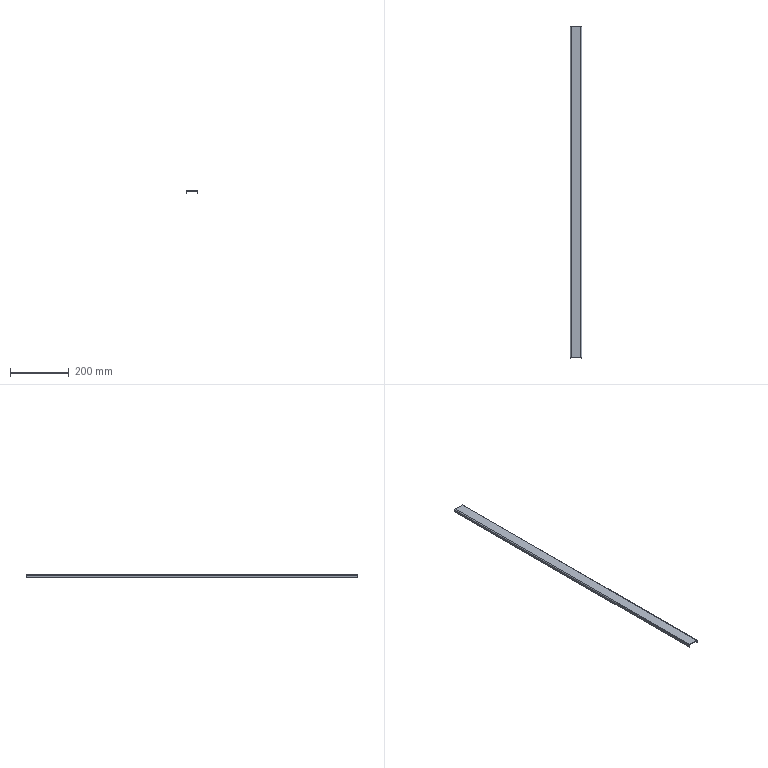Part | SolidWorks | features BaseBody 1 | 1 solid | 22 faces | box 40 x 1133 x 10 mm | volume 151532 mm3 | plane 18 | cylinder 4 | commonest cylinder face diameters 1 x2 6 x2
STEP:
#1=CARTESIAN_POINT('',(-17.5,566.5,-10.));
#2=VERTEX_POINT('',#1);
#3=CARTESIAN_POINT('',(-17.5,-566.5,-10.));
#4=VERTEX_POINT('',#3);
#5=CARTESIAN_POINT('',(-17.5,-566.5,-10.));
#6=DIRECTION('',(0.,-1.,0.));
#7=VECTOR('',#6,1000.);
#8=LINE('',#5,#7);
#9=EDGE_CURVE('',#2,#4,#8,.T.);
#10=ORIENTED_EDGE('',*,*,#9,.T.);
#11=CARTESIAN_POINT('',(-20.,-566.5,-10.));
#12=VERTEX_POINT('',#11);
#13=CARTESIAN_POINT('',(-20.,-566.5,-10.));
#14=DIRECTION('',(1.,0.,0.));
#15=VECTOR('',#14,1000.);
#16=LINE('',#13,#15);
#17=EDGE_CURVE('',#12,#4,#16,.T.);
#18=ORIENTED_EDGE('',*,*,#17,.F.);
#19=CARTESIAN_POINT('',(-20.,566.5,-10.));
#20=VERTEX_POINT('',#19);
#21=CARTESIAN_POINT('',(-20.,0.,-10.));
#22=DIRECTION('',(0.,-1.,0.));
#23=VECTOR('',#22,1000.);
#24=LINE('',#21,#23);
#25=EDGE_CURVE('',#20,#12,#24,.T.);
#26=ORIENTED_EDGE('',*,*,#25,.F.);
#27=CARTESIAN_POINT('',(-20.,566.5,-10.));
#28=DIRECTION('',(1.,0.,0.));
#29=VECTOR('',#28,1000.);
#30=LINE('',#27,#29);
#31=EDGE_CURVE('',#20,#2,#30,.T.);
#32=ORIENTED_EDGE('',*,*,#31,.T.);
#33=EDGE_LOOP('',(#10,#18,#26,#32));
#34=FACE_OUTER_BOUND('',#33,.T.);
#35=CARTESIAN_POINT('',(-20.,-566.5,-10.));
#36=DIRECTION('',(0.,0.,1.));
#37=DIRECTION('',(1.,0.,0.));
#38=AXIS2_PLACEMENT_3D('',#35,#36,#37);
#39=PLANE('',#38);
#40=ADVANCED_FACE('',(#34),#39,.F.);
#41=CARTESIAN_POINT('',(-17.5,566.5,-3.));
#42=VERTEX_POINT('',#41);
#43=CARTESIAN_POINT('',(-17.5,566.5,-10.));
#44=DIRECTION('',(0.,0.,-1.));
#45=VECTOR('',#44,1000.);
#46=LINE('',#43,#45);
#47=EDGE_CURVE('',#42,#2,#46,.T.);
#48=ORIENTED_EDGE('',*,*,#47,.F.);
#49=CARTESIAN_POINT('',(-17.5,-566.5,-3.));
#50=VERTEX_POINT('',#49);
#51=CARTESIAN_POINT('',(-17.5,-566.5,-3.));
#52=DIRECTION('',(0.,1.,0.));
#53=VECTOR('',#52,1000.);
#54=LINE('',#51,#53);
#55=EDGE_CURVE('',#50,#42,#54,.T.);
#56=ORIENTED_EDGE('',*,*,#55,.F.);
#57=CARTESIAN_POINT('',(-17.5,-566.5,-2.5));
#58=DIRECTION('',(0.,0.,1.));
#59=VECTOR('',#58,1000.);
#60=LINE('',#57,#59);
#61=EDGE_CURVE('',#4,#50,#60,.T.);
#62=ORIENTED_EDGE('',*,*,#61,.F.);
#63=ORIENTED_EDGE('',*,*,#9,.F.);
#64=EDGE_LOOP('',(#48,#56,#62,#63));
#65=FACE_OUTER_BOUND('',#64,.T.);
#66=CARTESIAN_POINT('',(-17.5,0.,0.));
#67=DIRECTION('',(1.,0.,0.));
#68=DIRECTION('',(0.,0.,-1.));
#69=AXIS2_PLACEMENT_3D('',#66,#67,#68);
#70=PLANE('',#69);
#71=ADVANCED_FACE('',(#65),#70,.T.);
#72=CARTESIAN_POINT('',(-20.,566.5,-3.));
#73=VERTEX_POINT('',#72);
#74=CARTESIAN_POINT('',(-20.,-566.5,-3.));
#75=VERTEX_POINT('',#74);
#76=CARTESIAN_POINT('',(-20.,-566.5,-3.));
#77=DIRECTION('',(0.,-1.,0.));
#78=VECTOR('',#77,1000.);
#79=LINE('',#76,#78);
#80=EDGE_CURVE('',#73,#75,#79,.T.);
#81=ORIENTED_EDGE('',*,*,#80,.F.);
#82=CARTESIAN_POINT('',(-20.,566.5,0.));
#83=DIRECTION('',(0.,0.,-1.));
#84=VECTOR('',#83,1000.);
#85=LINE('',#82,#84);
#86=EDGE_CURVE('',#73,#20,#85,.T.);
#87=ORIENTED_EDGE('',*,*,#86,.T.);
#88=ORIENTED_EDGE('',*,*,#25,.T.);
#89=CARTESIAN_POINT('',(-20.,-566.5,0.));
#90=DIRECTION('',(0.,0.,1.));
#91=VECTOR('',#90,1000.);
#92=LINE('',#89,#91);
#93=EDGE_CURVE('',#12,#75,#92,.T.);
#94=ORIENTED_EDGE('',*,*,#93,.T.);
#95=EDGE_LOOP('',(#81,#87,#88,#94));
#96=FACE_OUTER_BOUND('',#95,.T.);
#97=CARTESIAN_POINT('',(-20.,0.,0.));
#98=DIRECTION('',(1.,0.,0.));
#99=DIRECTION('',(0.,0.,-1.));
#100=AXIS2_PLACEMENT_3D('',#97,#98,#99);
#101=PLANE('',#100);
#102=ADVANCED_FACE('',(#96),#101,.F.);
#103=CARTESIAN_POINT('',(-20.,-566.5,-3.));
#104=DIRECTION('',(-1.,0.,0.));
#105=VECTOR('',#104,1000.);
#106=LINE('',#103,#105);
#107=EDGE_CURVE('',#50,#75,#106,.T.);
#108=ORIENTED_EDGE('',*,*,#107,.T.);
#109=ORIENTED_EDGE('',*,*,#93,.F.);
#110=ORIENTED_EDGE('',*,*,#17,.T.);
#111=ORIENTED_EDGE('',*,*,#61,.T.);
#112=EDGE_LOOP('',(#108,#109,#110,#111));
#113=FACE_OUTER_BOUND('',#112,.T.);
#114=CARTESIAN_POINT('',(-20.,-566.5,-2.5));
#115=DIRECTION('',(0.,1.,0.));
#116=DIRECTION('',(0.,0.,-1.));
#117=AXIS2_PLACEMENT_3D('',#114,#115,#116);
#118=PLANE('',#117);
#119=ADVANCED_FACE('',(#113),#118,.F.);
#120=CARTESIAN_POINT('',(-17.5,566.5,-3.));
#121=DIRECTION('',(-1.,0.,0.));
#122=VECTOR('',#121,1000.);
#123=LINE('',#120,#122);
#124=EDGE_CURVE('',#42,#73,#123,.T.);
#125=ORIENTED_EDGE('',*,*,#124,.F.);
#126=ORIENTED_EDGE('',*,*,#47,.T.);
#127=ORIENTED_EDGE('',*,*,#31,.F.);
#128=ORIENTED_EDGE('',*,*,#86,.F.);
#129=EDGE_LOOP('',(#125,#126,#127,#128));
#130=FACE_OUTER_BOUND('',#129,.T.);
#131=CARTESIAN_POINT('',(-20.,566.5,-10.));
#132=DIRECTION('',(0.,-1.,0.));
#133=DIRECTION('',(0.,0.,-1.));
#134=AXIS2_PLACEMENT_3D('',#131,#132,#133);
#135=PLANE('',#134);
#136=ADVANCED_FACE('',(#130),#135,.F.);
#137=CARTESIAN_POINT('',(-17.,566.5,-2.5));
#138=VERTEX_POINT('',#137);
#139=CARTESIAN_POINT('',(-17.,-566.5,-2.5));
#140=VERTEX_POINT('',#139);
#141=CARTESIAN_POINT('',(-17.,566.5,-2.5));
#142=DIRECTION('',(0.,-1.,0.));
#143=VECTOR('',#142,1000.);
#144=LINE('',#141,#143);
#145=EDGE_CURVE('',#138,#140,#144,.T.);
#146=ORIENTED_EDGE('',*,*,#145,.T.);
#147=CARTESIAN_POINT('',(-17.,-566.5,-3.));
#148=DIRECTION('',(0.,-1.,0.));
#149=DIRECTION('',(0.,0.,1.));
#150=AXIS2_PLACEMENT_3D('',#147,#148,#149);
#151=CIRCLE('',#150,0.5);
#152=EDGE_CURVE('',#140,#50,#151,.T.);
#153=ORIENTED_EDGE('',*,*,#152,.T.);
#154=ORIENTED_EDGE('',*,*,#55,.T.);
#155=CARTESIAN_POINT('',(-17.,566.5,-3.));
#156=DIRECTION('',(0.,1.,0.));
#157=DIRECTION('',(0.,0.,1.));
#158=AXIS2_PLACEMENT_3D('',#155,#156,#157);
#159=CIRCLE('',#158,0.5);
#160=EDGE_CURVE('',#42,#138,#159,.T.);
#161=ORIENTED_EDGE('',*,*,#160,.T.);
#162=EDGE_LOOP('',(#146,#153,#154,#161));
#163=FACE_OUTER_BOUND('',#162,.T.);
#164=CARTESIAN_POINT('',(-17.,566.5,-3.));
#165=DIRECTION('',(0.,1.,0.));
#166=DIRECTION('',(-1.,0.,0.));
#167=AXIS2_PLACEMENT_3D('',#164,#165,#166);
#168=CYLINDRICAL_SURFACE('',#167,0.5);
#169=ADVANCED_FACE('',(#163),#168,.F.);
#170=CARTESIAN_POINT('',(-17.,566.5,0.));
#171=VERTEX_POINT('',#170);
#172=CARTESIAN_POINT('',(-17.,-566.5,0.));
#173=VERTEX_POINT('',#172);
#174=CARTESIAN_POINT('',(-17.,566.5,0.));
#175=DIRECTION('',(0.,-1.,0.));
#176=VECTOR('',#175,1000.);
#177=LINE('',#174,#176);
#178=EDGE_CURVE('',#171,#173,#177,.T.);
#179=ORIENTED_EDGE('',*,*,#178,.F.);
#180=CARTESIAN_POINT('',(-17.,566.5,-3.));
#181=DIRECTION('',(0.,1.,0.));
#182=DIRECTION('',(0.,0.,1.));
#183=AXIS2_PLACEMENT_3D('',#180,#181,#182);
#184=CIRCLE('',#183,3.);
#185=EDGE_CURVE('',#73,#171,#184,.T.);
#186=ORIENTED_EDGE('',*,*,#185,.F.);
#187=ORIENTED_EDGE('',*,*,#80,.T.);
#188=CARTESIAN_POINT('',(-17.,-566.5,-3.));
#189=DIRECTION('',(0.,-1.,0.));
#190=DIRECTION('',(0.,0.,1.));
#191=AXIS2_PLACEMENT_3D('',#188,#189,#190);
#192=CIRCLE('',#191,3.);
#193=EDGE_CURVE('',#173,#75,#192,.T.);
#194=ORIENTED_EDGE('',*,*,#193,.F.);
#195=EDGE_LOOP('',(#179,#186,#187,#194));
#196=FACE_OUTER_BOUND('',#195,.T.);
#197=CARTESIAN_POINT('',(-17.,566.5,-3.));
#198=DIRECTION('',(0.,1.,0.));
#199=DIRECTION('',(-1.,0.,0.));
#200=AXIS2_PLACEMENT_3D('',#197,#198,#199);
#201=CYLINDRICAL_SURFACE('',#200,3.);
#202=ADVANCED_FACE('',(#196),#201,.T.);
#203=ORIENTED_EDGE('',*,*,#160,.F.);
#204=ORIENTED_EDGE('',*,*,#124,.T.);
#205=ORIENTED_EDGE('',*,*,#185,.T.);
#206=CARTESIAN_POINT('',(-17.,566.5,-2.5));
#207=DIRECTION('',(0.,0.,1.));
#208=VECTOR('',#207,1000.);
#209=LINE('',#206,#208);
#210=EDGE_CURVE('',#138,#171,#209,.T.);
#211=ORIENTED_EDGE('',*,*,#210,.F.);
#212=EDGE_LOOP('',(#203,#204,#205,#211));
#213=FACE_OUTER_BOUND('',#212,.T.);
#214=CARTESIAN_POINT('',(-17.,566.5,-3.));
#215=DIRECTION('',(0.,-1.,0.));
#216=DIRECTION('',(0.,0.,-1.));
#217=AXIS2_PLACEMENT_3D('',#214,#215,#216);
#218=PLANE('',#217);
#219=ADVANCED_FACE('',(#213),#218,.F.);
#220=ORIENTED_EDGE('',*,*,#107,.F.);
#221=ORIENTED_EDGE('',*,*,#152,.F.);
#222=CARTESIAN_POINT('',(-17.,-566.5,-2.5));
#223=DIRECTION('',(0.,0.,1.));
#224=VECTOR('',#223,1000.);
#225=LINE('',#222,#224);
#226=EDGE_CURVE('',#140,#173,#225,.T.);
#227=ORIENTED_EDGE('',*,*,#226,.T.);
#228=ORIENTED_EDGE('',*,*,#193,.T.);
#229=EDGE_LOOP('',(#220,#221,#227,#228));
#230=FACE_OUTER_BOUND('',#229,.T.);
#231=CARTESIAN_POINT('',(-17.,-566.5,-3.));
#232=DIRECTION('',(0.,-1.,0.));
#233=DIRECTION('',(0.,0.,-1.));
#234=AXIS2_PLACEMENT_3D('',#231,#232,#233);
#235=PLANE('',#234);
#236=ADVANCED_FACE('',(#230),#235,.T.);
#237=CARTESIAN_POINT('',(17.5,-566.5,-10.));
#238=VERTEX_POINT('',#237);
#239=CARTESIAN_POINT('',(17.5,566.5,-10.));
#240=VERTEX_POINT('',#239);
#241=CARTESIAN_POINT('',(17.5,566.5,-10.));
#242=DIRECTION('',(0.,1.,0.));
#243=VECTOR('',#242,1000.);
#244=LINE('',#241,#243);
#245=EDGE_CURVE('',#238,#240,#244,.T.);
#246=ORIENTED_EDGE('',*,*,#245,.T.);
#247=CARTESIAN_POINT('',(20.,566.5,-10.));
#248=VERTEX_POINT('',#247);
#249=CARTESIAN_POINT('',(20.,566.5,-10.));
#250=DIRECTION('',(-1.,0.,0.));
#251=VECTOR('',#250,1000.);
#252=LINE('',#249,#251);
#253=EDGE_CURVE('',#248,#240,#252,.T.);
#254=ORIENTED_EDGE('',*,*,#253,.F.);
#255=CARTESIAN_POINT('',(20.,-566.5,-10.));
#256=VERTEX_POINT('',#255);
#257=CARTESIAN_POINT('',(20.,0.,-10.));
#258=DIRECTION('',(0.,1.,0.));
#259=VECTOR('',#258,1000.);
#260=LINE('',#257,#259);
#261=EDGE_CURVE('',#256,#248,#260,.T.);
#262=ORIENTED_EDGE('',*,*,#261,.F.);
#263=CARTESIAN_POINT('',(20.,-566.5,-10.));
#264=DIRECTION('',(-1.,0.,0.));
#265=VECTOR('',#264,1000.);
#266=LINE('',#263,#265);
#267=EDGE_CURVE('',#256,#238,#266,.T.);
#268=ORIENTED_EDGE('',*,*,#267,.T.);
#269=EDGE_LOOP('',(#246,#254,#262,#268));
#270=FACE_OUTER_BOUND('',#269,.T.);
#271=CARTESIAN_POINT('',(20.,566.5,-10.));
#272=DIRECTION('',(0.,0.,1.));
#273=DIRECTION('',(1.,0.,0.));
#274=AXIS2_PLACEMENT_3D('',#271,#272,#273);
#275=PLANE('',#274);
#276=ADVANCED_FACE('',(#270),#275,.F.);
#277=CARTESIAN_POINT('',(17.5,-566.5,-3.));
#278=VERTEX_POINT('',#277);
#279=CARTESIAN_POINT('',(17.5,-566.5,-10.));
#280=DIRECTION('',(0.,0.,-1.));
#281=VECTOR('',#280,1000.);
#282=LINE('',#279,#281);
#283=EDGE_CURVE('',#278,#238,#282,.T.);
#284=ORIENTED_EDGE('',*,*,#283,.F.);
#285=CARTESIAN_POINT('',(17.5,566.5,-3.));
#286=VERTEX_POINT('',#285);
#287=CARTESIAN_POINT('',(17.5,566.5,-3.));
#288=DIRECTION('',(0.,-1.,0.));
#289=VECTOR('',#288,1000.);
#290=LINE('',#287,#289);
#291=EDGE_CURVE('',#286,#278,#290,.T.);
#292=ORIENTED_EDGE('',*,*,#291,.F.);
#293=CARTESIAN_POINT('',(17.5,566.5,-2.5));
#294=DIRECTION('',(0.,0.,1.));
#295=VECTOR('',#294,1000.);
#296=LINE('',#293,#295);
#297=EDGE_CURVE('',#240,#286,#296,.T.);
#298=ORIENTED_EDGE('',*,*,#297,.F.);
#299=ORIENTED_EDGE('',*,*,#245,.F.);
#300=EDGE_LOOP('',(#284,#292,#298,#299));
#301=FACE_OUTER_BOUND('',#300,.T.);
#302=CARTESIAN_POINT('',(17.5,0.,0.));
#303=DIRECTION('',(-1.,0.,0.));
#304=DIRECTION('',(0.,0.,1.));
#305=AXIS2_PLACEMENT_3D('',#302,#303,#304);
#306=PLANE('',#305);
#307=ADVANCED_FACE('',(#301),#306,.T.);
#308=CARTESIAN_POINT('',(20.,-566.5,-3.));
#309=VERTEX_POINT('',#308);
#310=CARTESIAN_POINT('',(20.,566.5,-3.));
#311=VERTEX_POINT('',#310);
#312=CARTESIAN_POINT('',(20.,566.5,-3.));
#313=DIRECTION('',(0.,1.,0.));
#314=VECTOR('',#313,1000.);
#315=LINE('',#312,#314);
#316=EDGE_CURVE('',#309,#311,#315,.T.);
#317=ORIENTED_EDGE('',*,*,#316,.F.);
#318=CARTESIAN_POINT('',(20.,-566.5,0.));
#319=DIRECTION('',(0.,0.,-1.));
#320=VECTOR('',#319,1000.);
#321=LINE('',#318,#320);
#322=EDGE_CURVE('',#309,#256,#321,.T.);
#323=ORIENTED_EDGE('',*,*,#322,.T.);
#324=ORIENTED_EDGE('',*,*,#261,.T.);
#325=CARTESIAN_POINT('',(20.,566.5,0.));
#326=DIRECTION('',(0.,0.,1.));
#327=VECTOR('',#326,1000.);
#328=LINE('',#325,#327);
#329=EDGE_CURVE('',#248,#311,#328,.T.);
#330=ORIENTED_EDGE('',*,*,#329,.T.);
#331=EDGE_LOOP('',(#317,#323,#324,#330));
#332=FACE_OUTER_BOUND('',#331,.T.);
#333=CARTESIAN_POINT('',(20.,0.,0.));
#334=DIRECTION('',(-1.,0.,0.));
#335=DIRECTION('',(0.,0.,1.));
#336=AXIS2_PLACEMENT_3D('',#333,#334,#335);
#337=PLANE('',#336);
#338=ADVANCED_FACE('',(#332),#337,.F.);
#339=CARTESIAN_POINT('',(20.,566.5,-3.));
#340=DIRECTION('',(1.,0.,0.));
#341=VECTOR('',#340,1000.);
#342=LINE('',#339,#341);
#343=EDGE_CURVE('',#286,#311,#342,.T.);
#344=ORIENTED_EDGE('',*,*,#343,.T.);
#345=ORIENTED_EDGE('',*,*,#329,.F.);
#346=ORIENTED_EDGE('',*,*,#253,.T.);
#347=ORIENTED_EDGE('',*,*,#297,.T.);
#348=EDGE_LOOP('',(#344,#345,#346,#347));
#349=FACE_OUTER_BOUND('',#348,.T.);
#350=CARTESIAN_POINT('',(20.,566.5,-2.5));
#351=DIRECTION('',(0.,-1.,0.));
#352=DIRECTION('',(0.,0.,-1.));
#353=AXIS2_PLACEMENT_3D('',#350,#351,#352);
#354=PLANE('',#353);
#355=ADVANCED_FACE('',(#349),#354,.F.);
#356=CARTESIAN_POINT('',(17.5,-566.5,-3.));
#357=DIRECTION('',(1.,0.,0.));
#358=VECTOR('',#357,1000.);
#359=LINE('',#356,#358);
#360=EDGE_CURVE('',#278,#309,#359,.T.);
#361=ORIENTED_EDGE('',*,*,#360,.F.);
#362=ORIENTED_EDGE('',*,*,#283,.T.);
#363=ORIENTED_EDGE('',*,*,#267,.F.);
#364=ORIENTED_EDGE('',*,*,#322,.F.);
#365=EDGE_LOOP('',(#361,#362,#363,#364));
#366=FACE_OUTER_BOUND('',#365,.T.);
#367=CARTESIAN_POINT('',(20.,-566.5,-10.));
#368=DIRECTION('',(0.,1.,0.));
#369=DIRECTION('',(0.,0.,-1.));
#370=AXIS2_PLACEMENT_3D('',#367,#368,#369);
#371=PLANE('',#370);
#372=ADVANCED_FACE('',(#366),#371,.F.);
#373=CARTESIAN_POINT('',(17.,-566.5,-2.5));
#374=VERTEX_POINT('',#373);
#375=CARTESIAN_POINT('',(17.,566.5,-2.5));
#376=VERTEX_POINT('',#375);
#377=CARTESIAN_POINT('',(17.,-566.5,-2.5));
#378=DIRECTION('',(0.,1.,0.));
#379=VECTOR('',#378,1000.);
#380=LINE('',#377,#379);
#381=EDGE_CURVE('',#374,#376,#380,.T.);
#382=ORIENTED_EDGE('',*,*,#381,.T.);
#383=CARTESIAN_POINT('',(17.,566.5,-3.));
#384=DIRECTION('',(0.,1.,0.));
#385=DIRECTION('',(0.,0.,-1.));
#386=AXIS2_PLACEMENT_3D('',#383,#384,#385);
#387=CIRCLE('',#386,0.5);
#388=EDGE_CURVE('',#376,#286,#387,.T.);
#389=ORIENTED_EDGE('',*,*,#388,.T.);
#390=ORIENTED_EDGE('',*,*,#291,.T.);
#391=CARTESIAN_POINT('',(17.,-566.5,-3.));
#392=DIRECTION('',(0.,-1.,0.));
#393=DIRECTION('',(0.,0.,-1.));
#394=AXIS2_PLACEMENT_3D('',#391,#392,#393);
#395=CIRCLE('',#394,0.5);
#396=EDGE_CURVE('',#278,#374,#395,.T.);
#397=ORIENTED_EDGE('',*,*,#396,.T.);
#398=EDGE_LOOP('',(#382,#389,#390,#397));
#399=FACE_OUTER_BOUND('',#398,.T.);
#400=CARTESIAN_POINT('',(17.,-566.5,-3.));
#401=DIRECTION('',(0.,-1.,0.));
#402=DIRECTION('',(1.,0.,0.));
#403=AXIS2_PLACEMENT_3D('',#400,#401,#402);
#404=CYLINDRICAL_SURFACE('',#403,0.5);
#405=ADVANCED_FACE('',(#399),#404,.F.);
#406=CARTESIAN_POINT('',(17.,-566.5,0.));
#407=VERTEX_POINT('',#406);
#408=CARTESIAN_POINT('',(17.,566.5,0.));
#409=VERTEX_POINT('',#408);
#410=CARTESIAN_POINT('',(17.,-566.5,0.));
#411=DIRECTION('',(0.,1.,0.));
#412=VECTOR('',#411,1000.);
#413=LINE('',#410,#412);
#414=EDGE_CURVE('',#407,#409,#413,.T.);
#415=ORIENTED_EDGE('',*,*,#414,.F.);
#416=CARTESIAN_POINT('',(17.,-566.5,-3.));
#417=DIRECTION('',(0.,-1.,0.));
#418=DIRECTION('',(0.,0.,-1.));
#419=AXIS2_PLACEMENT_3D('',#416,#417,#418);
#420=CIRCLE('',#419,3.);
#421=EDGE_CURVE('',#309,#407,#420,.T.);
#422=ORIENTED_EDGE('',*,*,#421,.F.);
#423=ORIENTED_EDGE('',*,*,#316,.T.);
#424=CARTESIAN_POINT('',(17.,566.5,-3.));
#425=DIRECTION('',(0.,1.,0.));
#426=DIRECTION('',(0.,0.,-1.));
#427=AXIS2_PLACEMENT_3D('',#424,#425,#426);
#428=CIRCLE('',#427,3.);
#429=EDGE_CURVE('',#409,#311,#428,.T.);
#430=ORIENTED_EDGE('',*,*,#429,.F.);
#431=EDGE_LOOP('',(#415,#422,#423,#430));
#432=FACE_OUTER_BOUND('',#431,.T.);
#433=CARTESIAN_POINT('',(17.,-566.5,-3.));
#434=DIRECTION('',(0.,-1.,0.));
#435=DIRECTION('',(1.,0.,0.));
#436=AXIS2_PLACEMENT_3D('',#433,#434,#435);
#437=CYLINDRICAL_SURFACE('',#436,3.);
#438=ADVANCED_FACE('',(#432),#437,.T.);
#439=ORIENTED_EDGE('',*,*,#396,.F.);
#440=ORIENTED_EDGE('',*,*,#360,.T.);
#441=ORIENTED_EDGE('',*,*,#421,.T.);
#442=CARTESIAN_POINT('',(17.,-566.5,-2.5));
#443=DIRECTION('',(0.,0.,1.));
#444=VECTOR('',#443,1000.);
#445=LINE('',#442,#444);
#446=EDGE_CURVE('',#374,#407,#445,.T.);
#447=ORIENTED_EDGE('',*,*,#446,.F.);
#448=EDGE_LOOP('',(#439,#440,#441,#447));
#449=FACE_OUTER_BOUND('',#448,.T.);
#450=CARTESIAN_POINT('',(17.,-566.5,-3.));
#451=DIRECTION('',(0.,1.,0.));
#452=DIRECTION('',(1.,0.,0.));
#453=AXIS2_PLACEMENT_3D('',#450,#451,#452);
#454=PLANE('',#453);
#455=ADVANCED_FACE('',(#449),#454,.F.);
#456=ORIENTED_EDGE('',*,*,#343,.F.);
#457=ORIENTED_EDGE('',*,*,#388,.F.);
#458=CARTESIAN_POINT('',(17.,566.5,-2.5));
#459=DIRECTION('',(0.,0.,1.));
#460=VECTOR('',#459,1000.);
#461=LINE('',#458,#460);
#462=EDGE_CURVE('',#376,#409,#461,.T.);
#463=ORIENTED_EDGE('',*,*,#462,.T.);
#464=ORIENTED_EDGE('',*,*,#429,.T.);
#465=EDGE_LOOP('',(#456,#457,#463,#464));
#466=FACE_OUTER_BOUND('',#465,.T.);
#467=CARTESIAN_POINT('',(17.,566.5,-3.));
#468=DIRECTION('',(0.,1.,0.));
#469=DIRECTION('',(1.,0.,0.));
#470=AXIS2_PLACEMENT_3D('',#467,#468,#469);
#471=PLANE('',#470);
#472=ADVANCED_FACE('',(#466),#471,.T.);
#473=ORIENTED_EDGE('',*,*,#226,.F.);
#474=CARTESIAN_POINT('',(20.,-566.5,-2.5));
#475=DIRECTION('',(1.,0.,0.));
#476=VECTOR('',#475,1000.);
#477=LINE('',#474,#476);
#478=EDGE_CURVE('',#140,#374,#477,.T.);
#479=ORIENTED_EDGE('',*,*,#478,.T.);
#480=ORIENTED_EDGE('',*,*,#446,.T.);
#481=CARTESIAN_POINT('',(20.,-566.5,0.));
#482=DIRECTION('',(1.,0.,0.));
#483=VECTOR('',#482,1000.);
#484=LINE('',#481,#483);
#485=EDGE_CURVE('',#173,#407,#484,.T.);
#486=ORIENTED_EDGE('',*,*,#485,.F.);
#487=EDGE_LOOP('',(#473,#479,#480,#486));
#488=FACE_OUTER_BOUND('',#487,.T.);
#489=CARTESIAN_POINT('',(20.,-566.5,-2.5));
#490=DIRECTION('',(0.,-1.,0.));
#491=DIRECTION('',(0.,0.,-1.));
#492=AXIS2_PLACEMENT_3D('',#489,#490,#491);
#493=PLANE('',#492);
#494=ADVANCED_FACE('',(#488),#493,.T.);
#495=CARTESIAN_POINT('',(20.,566.5,-2.5));
#496=DIRECTION('',(-1.,0.,0.));
#497=VECTOR('',#496,1000.);
#498=LINE('',#495,#497);
#499=EDGE_CURVE('',#376,#138,#498,.T.);
#500=ORIENTED_EDGE('',*,*,#499,.T.);
#501=ORIENTED_EDGE('',*,*,#210,.T.);
#502=CARTESIAN_POINT('',(20.,566.5,0.));
#503=DIRECTION('',(-1.,0.,0.));
#504=VECTOR('',#503,1000.);
#505=LINE('',#502,#504);
#506=EDGE_CURVE('',#409,#171,#505,.T.);
#507=ORIENTED_EDGE('',*,*,#506,.F.);
#508=ORIENTED_EDGE('',*,*,#462,.F.);
#509=EDGE_LOOP('',(#500,#501,#507,#508));
#510=FACE_OUTER_BOUND('',#509,.T.);
#511=CARTESIAN_POINT('',(20.,566.5,-2.5));
#512=DIRECTION('',(0.,1.,0.));
#513=DIRECTION('',(1.,0.,0.));
#514=AXIS2_PLACEMENT_3D('',#511,#512,#513);
#515=PLANE('',#514);
#516=ADVANCED_FACE('',(#510),#515,.T.);
#517=ORIENTED_EDGE('',*,*,#178,.T.);
#518=ORIENTED_EDGE('',*,*,#485,.T.);
#519=ORIENTED_EDGE('',*,*,#414,.T.);
#520=ORIENTED_EDGE('',*,*,#506,.T.);
#521=EDGE_LOOP('',(#517,#518,#519,#520));
#522=FACE_OUTER_BOUND('',#521,.T.);
#523=CARTESIAN_POINT('',(0.,0.,0.));
#524=DIRECTION('',(0.,0.,-1.));
#525=DIRECTION('',(0.,-1.,0.));
#526=AXIS2_PLACEMENT_3D('',#523,#524,#525);
#527=PLANE('',#526);
#528=ADVANCED_FACE('',(#522),#527,.F.);
#529=ORIENTED_EDGE('',*,*,#478,.F.);
#530=ORIENTED_EDGE('',*,*,#145,.F.);
#531=ORIENTED_EDGE('',*,*,#499,.F.);
#532=ORIENTED_EDGE('',*,*,#381,.F.);
#533=EDGE_LOOP('',(#529,#530,#531,#532));
#534=FACE_OUTER_BOUND('',#533,.T.);
#535=CARTESIAN_POINT('',(0.,0.,-2.5));
#536=DIRECTION('',(0.,0.,-1.));
#537=DIRECTION('',(0.,-1.,0.));
#538=AXIS2_PLACEMENT_3D('',#535,#536,#537);
#539=PLANE('',#538);
#540=ADVANCED_FACE('',(#534),#539,.T.);
#541=CLOSED_SHELL('',(#40,#71,#102,#119,#136,#169,#202,#219,#236,#276,#307,#338,#355,#372,#405,#438,#455,#472,#494,#516,#528,#540));
#542=MANIFOLD_SOLID_BREP('',#541);
#543=CARTESIAN_POINT('',(0.,0.,0.));
#544=DIRECTION('',(0.,0.,1.));
#545=DIRECTION('',(1.,0.,0.));
#546=AXIS2_PLACEMENT_3D('',#543,#544,#545);
#547=(LENGTH_UNIT()NAMED_UNIT(*)SI_UNIT(.MILLI.,.METRE.));
#548=UNCERTAINTY_MEASURE_WITH_UNIT(LENGTH_MEASURE(0.00001),#547,'','');
#549=(NAMED_UNIT(*)PLANE_ANGLE_UNIT()SI_UNIT($,.RADIAN.));
#550=(NAMED_UNIT(*)SI_UNIT($,.STERADIAN.)SOLID_ANGLE_UNIT());
#551=(GEOMETRIC_REPRESENTATION_CONTEXT(3)GLOBAL_UNCERTAINTY_ASSIGNED_CONTEXT((#548))GLOBAL_UNIT_ASSIGNED_CONTEXT((#547,#549,#550))REPRESENTATION_CONTEXT('',''));
#552=ADVANCED_BREP_SHAPE_REPRESENTATION('',(#542,#546),#551);